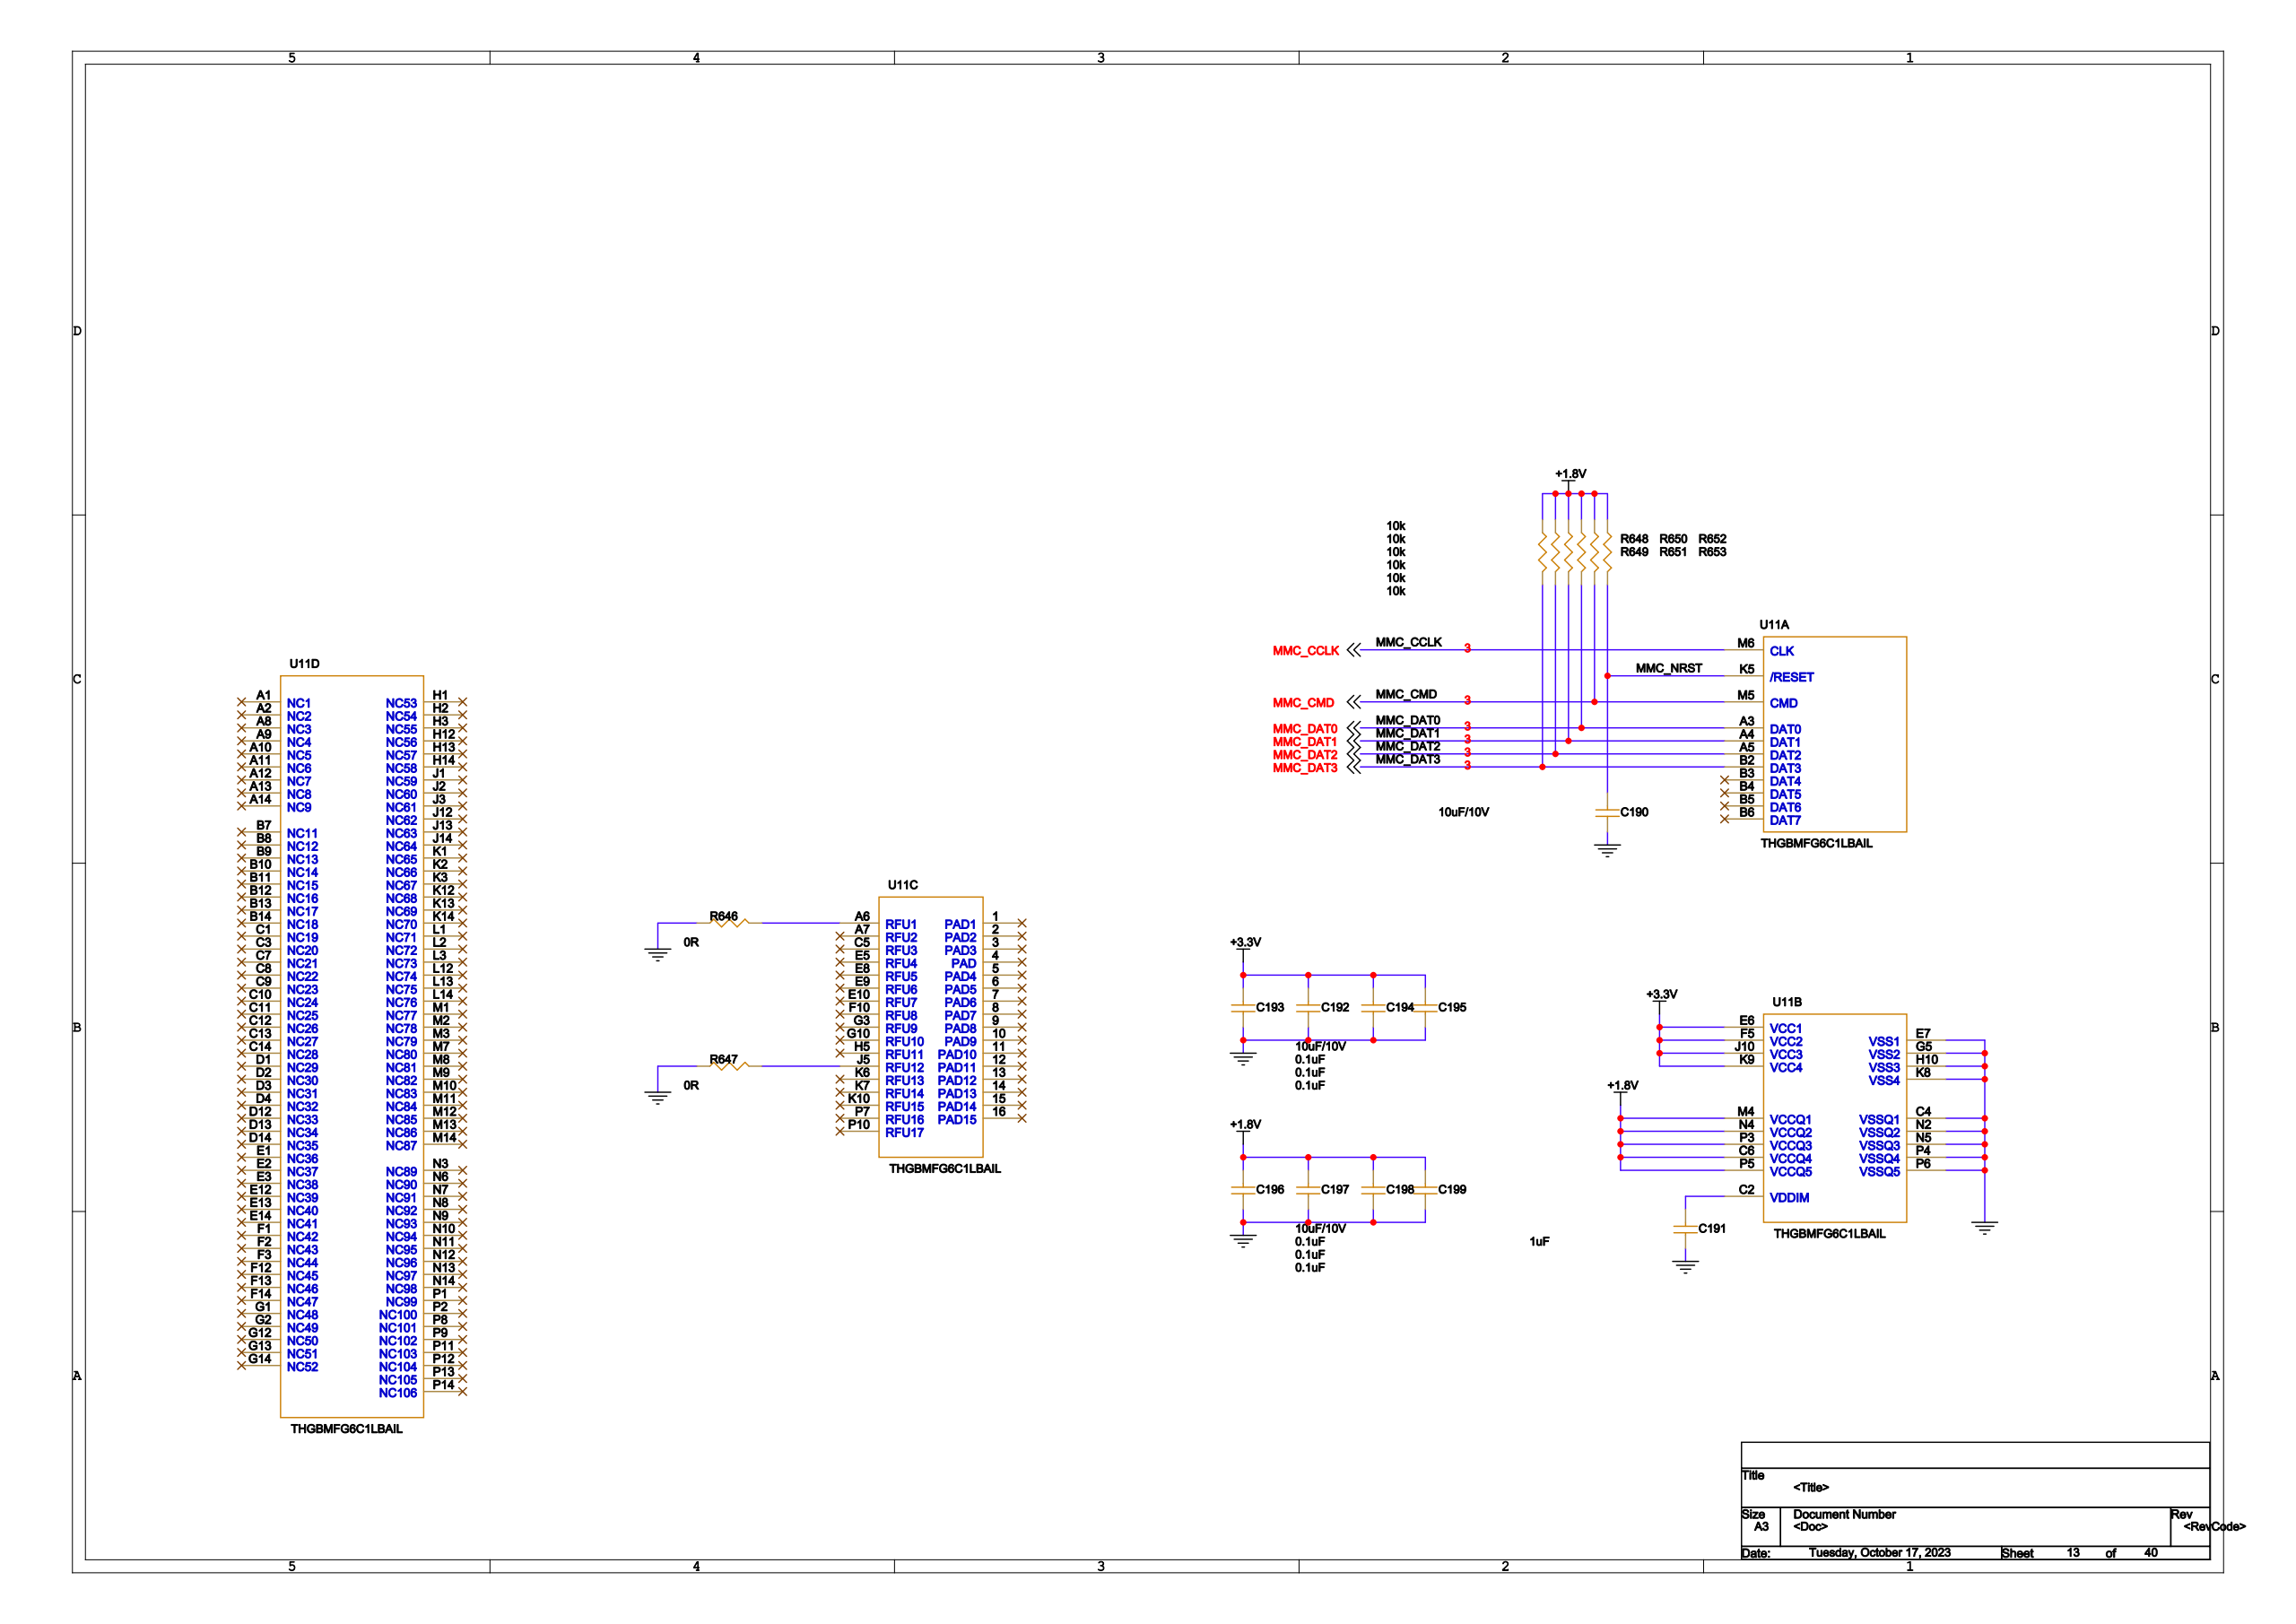Circuit board | Cadence Allegro | 1793 parts | 1223 nets | one sheet of the schematic
Parts on this sheet (reference | value | footprint):
C190 | 10uF/10V | C0402
C191 | 1uF | C0402
C192 | 0.1uF | C0402
C193 | 10uF/10V | C0402
C194 | 0.1uF | C0402
C195 | 0.1uF | C0402
C196 | 10uF/10V | C0402
C197 | 0.1uF | C0402
C198 | 0.1uF | C0402
C199 | 0.1uF | C0402
R646 | 0R | R0402
R647 | 0R | R0402
R648 | 10k | R0402
R649 | 10k | R0402
R650 | 10k | R0402
R651 | 10k | R0402
R652 | 10k | R0402
R653 | 10k | R0402
U11 | THGBMFG6C1LBAIL | VFBGA
Nets of these parts (net: part-pin ...):
GND: C190-1 C191-1 C192-1 C193-1 C194-1 C195-1 C196-1 C197-1 C198-1 C199-1 R646-2 R647-2 U11-C4 U11-E7 U11-G5 U11-H10 U11-K8 U11-N2 U11-N5 U11-P4 U11-P6
+3.3V: C192-2 C193-2 C194-2 C195-2 U11-E6 U11-F5 U11-J10 U11-K9
+1.8V: C196-2 C197-2 C198-2 C199-2 R648-2 R649-2 R650-2 R651-2 R652-2 R653-2 U11-C6 U11-M4 U11-N4 U11-P3 U11-P5
N169302: C191-2 U11-C2
MMC_NRST: C190-2 R653-1 U11-K5
MMC_CCLK: U11-M6
MMC_DAT3: R648-1 U11-B2
MMC_DAT2: R649-1 U11-A5
MMC_DAT1: R650-1 U11-A4
MMC_DAT0: R651-1 U11-A3
MMC_CMD: R652-1 U11-M5
N167774: R646-1 U11-A6
N167804: R647-1 U11-J5